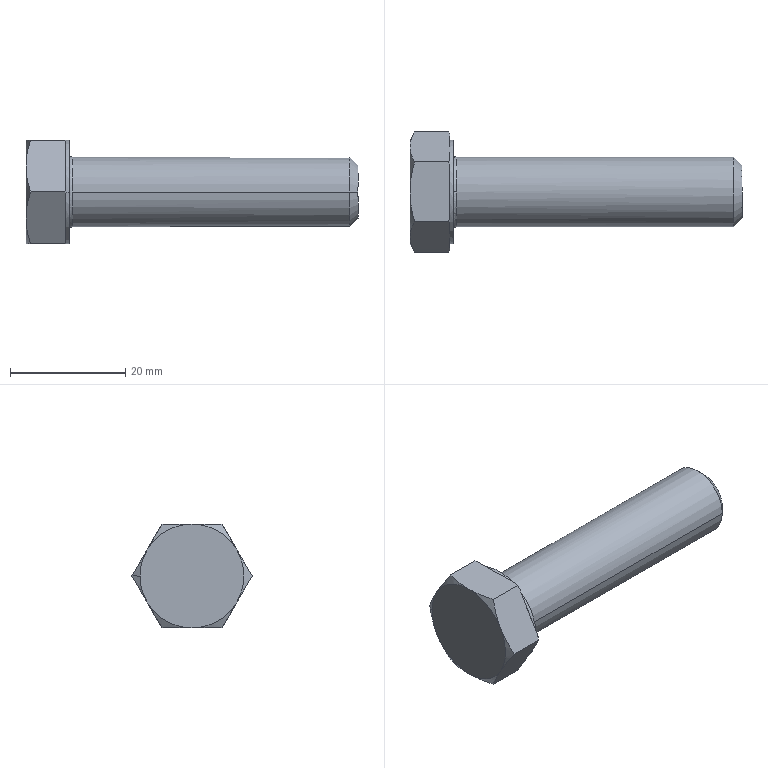Part | STEP file | 1 solid | 37 faces | box 57.5 x 20.785 x 18 mm | volume 7706 mm3 | cone 16 | plane 15 | cylinder 4 | spline 2 | commonest cylinder face diameters 12 x2 18 x2